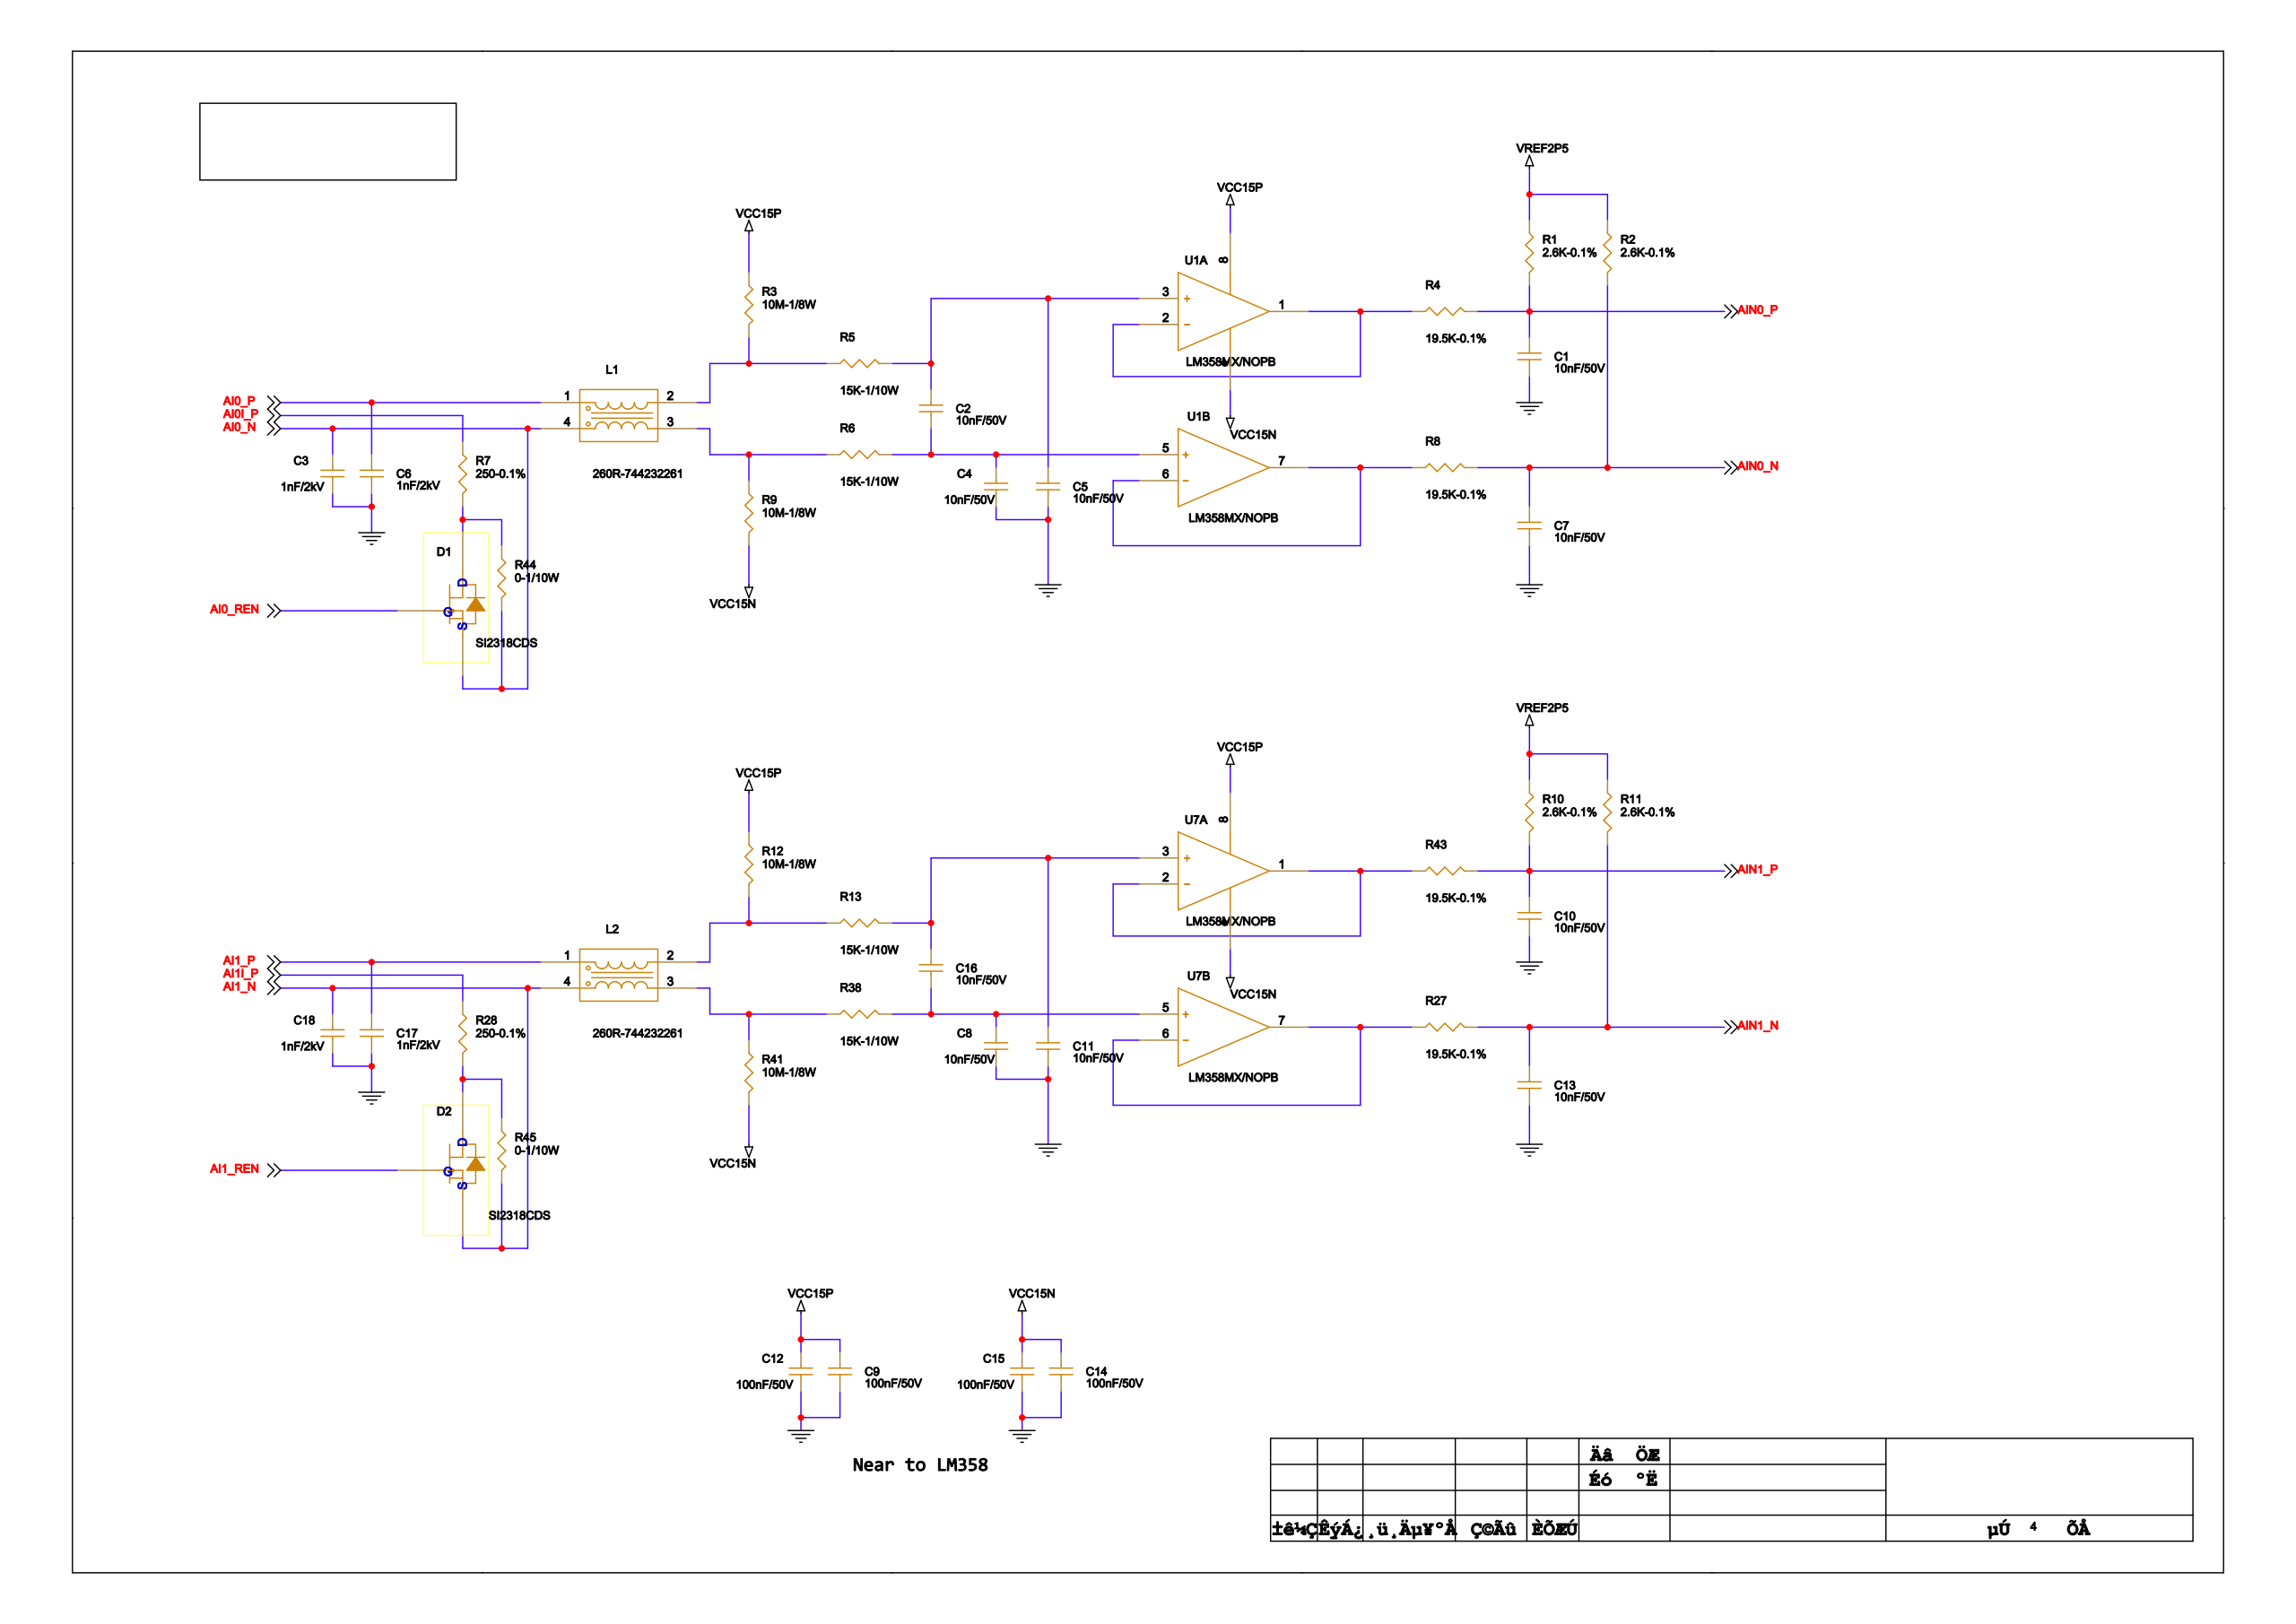Circuit board | Cadence Allegro | 65 parts | 41 nets | one sheet of the schematic
Parts on this sheet (reference | value | footprint):
C1 | 10nF/50V | C0603
C2 | 10nF/50V | C0603
C3 | 1nF/2kV | C1206
C4 | 10nF/50V | C0603
C5 | 10nF/50V | C0603
C6 | 1nF/2kV | C1206
C7 | 10nF/50V | C0603
C8 | 10nF/50V | C0603
C9 | 100nF/50V | C0603
C10 | 10nF/50V | C0603
C11 | 10nF/50V | C0603
C12 | 100nF/50V | C0603
C13 | 10nF/50V | C0603
C14 | 100nF/50V | C0603
C15 | 100nF/50V | C0603
C16 | 10nF/50V | C0603
C17 | 1nF/2kV | C1206
C18 | 1nF/2kV | C1206
D1 | SI2318CDS | SOT23
D2 | SI2318CDS | SOT23
L1 | 260R-744232261 | 744232261
L2 | 260R-744232261 | 744232261
R1 | 2.6K-0.1% | R0805
R2 | 2.6K-0.1% | R0805
R3 | 10M-1/8W | R0805
R4 | 19.5K-0.1% | R0805
R5 | 15K-1/10W | R0603
R6 | 15K-1/10W | R0603
R7 | 250-0.1% | R0805
R8 | 19.5K-0.1% | R0805
R9 | 10M-1/8W | R0805
R10 | 2.6K-0.1% | R0805
R11 | 2.6K-0.1% | R0805
R12 | 10M-1/8W | R0805
R13 | 15K-1/10W | R0603
R27 | 19.5K-0.1% | R0805
R28 | 250-0.1% | R0805
R38 | 15K-1/10W | R0603
R41 | 10M-1/8W | R0805
R43 | 19.5K-0.1% | R0805
R44 | 0-1/10W | R0603
R45 | 0-1/10W | R0603
Nets of these parts (net: part-pin ...):
AI0_N: C3-1 D1-2 L1-4 R44-2
AI0_REN: D1-1
N7790330: D1-3 R7-2 R44-1
AI1_N: C18-1 D2-2 L2-4 R45-2
AI1_REN: D2-1
N7793799: D2-3 R28-2 R45-1
AIN0_P: C1-1 R1-2 R4-2
GND: C1-2 C3-2 C4-2 C5-2 C6-2 C7-2 C8-2 C9-2 C10-2 C11-2 C12-2 C13-2 C14-2 C15-2 C17-2 C18-2
AIN1_P: C10-1 R10-2 R43-2
N7794115: C11-1 C16-1 R13-2
AIN1_N: C13-1 R11-2 R27-2
N7794091: C8-1 C16-2 R38-2
N7791236: C2-1 C5-1 R5-2
N7791207: C2-2 C4-1 R6-2
AIN0_N: C7-1 R2-2 R8-2
VCC15P: C9-1 C12-1 R3-1 R12-1
VCC15N: C14-1 C15-1 R9-2 R41-2
VREF2P5: R1-1 R2-1 R10-1 R11-1
AI1_P: C17-1 L2-1
AI0_P: C6-1 L1-1
AI1I_P: R28-1
AI0I_P: R7-1
N7790885: L1-2 R3-2 R5-1
N7790913: L1-3 R6-1 R9-1
N7794011: L2-2 R12-2 R13-1
N7794031: L2-3 R38-1 R41-1
N7794095: R27-1
N7791248: R4-1
N7794127: R43-1
N7791211: R8-1